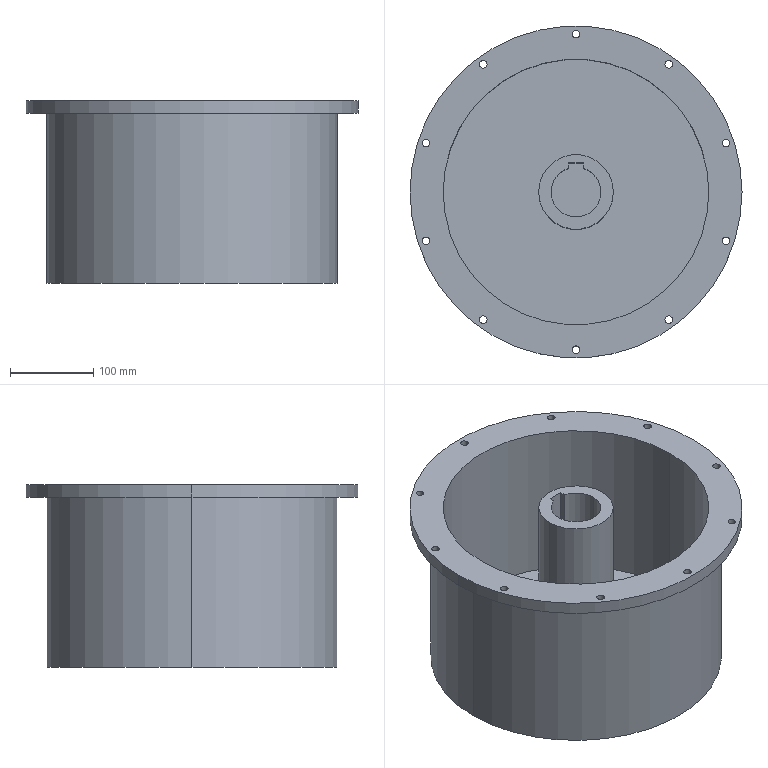Part | SolidWorks | features ICE 4, Extrusion 1 | 1 solid | 40 faces | box 400 x 400 x 220 mm | volume 6200986 mm3 | cylinder 31 | plane 9 | commonest cylinder face diameters 9 x20 60 x3 90 x2 320 x2 350 x2 400 x2
STEP:
#1=CARTESIAN_POINT('',(45.,0.,20.));
#2=VERTEX_POINT('',#1);
#3=CARTESIAN_POINT('',(-45.,0.,20.));
#4=VERTEX_POINT('',#3);
#5=CARTESIAN_POINT('',(0.,0.,20.));
#6=DIRECTION('',(0.,0.,1.));
#7=DIRECTION('',(1.,0.,0.));
#8=AXIS2_PLACEMENT_3D('',#5,#6,#7);
#9=CIRCLE('',#8,45.);
#10=EDGE_CURVE('',#2,#4,#9,.T.);
#11=ORIENTED_EDGE('',*,*,#10,.T.);
#12=CARTESIAN_POINT('',(-45.,0.,220.));
#13=VERTEX_POINT('',#12);
#14=CARTESIAN_POINT('',(-45.,0.,20.));
#15=DIRECTION('',(0.,0.,1.));
#16=VECTOR('',#15,1000.);
#17=LINE('',#14,#16);
#18=EDGE_CURVE('',#4,#13,#17,.T.);
#19=ORIENTED_EDGE('',*,*,#18,.T.);
#20=CARTESIAN_POINT('',(45.,0.,220.));
#21=VERTEX_POINT('',#20);
#22=CARTESIAN_POINT('',(0.,0.,220.));
#23=DIRECTION('',(0.,0.,1.));
#24=DIRECTION('',(1.,0.,0.));
#25=AXIS2_PLACEMENT_3D('',#22,#23,#24);
#26=CIRCLE('',#25,45.);
#27=EDGE_CURVE('',#21,#13,#26,.T.);
#28=ORIENTED_EDGE('',*,*,#27,.F.);
#29=CARTESIAN_POINT('',(45.,0.,20.));
#30=DIRECTION('',(0.,0.,1.));
#31=VECTOR('',#30,1000.);
#32=LINE('',#29,#31);
#33=EDGE_CURVE('',#2,#21,#32,.T.);
#34=ORIENTED_EDGE('',*,*,#33,.F.);
#35=EDGE_LOOP('',(#11,#19,#28,#34));
#36=FACE_OUTER_BOUND('',#35,.T.);
#37=CARTESIAN_POINT('',(0.,0.,20.));
#38=DIRECTION('',(0.,0.,1.));
#39=DIRECTION('',(1.,0.,0.));
#40=AXIS2_PLACEMENT_3D('',#37,#38,#39);
#41=CYLINDRICAL_SURFACE('',#40,45.);
#42=ADVANCED_FACE('',(#36),#41,.T.);
#43=CARTESIAN_POINT('',(-160.,0.,20.));
#44=VERTEX_POINT('',#43);
#45=CARTESIAN_POINT('',(160.,0.,20.));
#46=VERTEX_POINT('',#45);
#47=CARTESIAN_POINT('',(0.,0.,20.));
#48=DIRECTION('',(0.,0.,1.));
#49=DIRECTION('',(1.,0.,0.));
#50=AXIS2_PLACEMENT_3D('',#47,#48,#49);
#51=CIRCLE('',#50,160.);
#52=EDGE_CURVE('',#44,#46,#51,.T.);
#53=ORIENTED_EDGE('',*,*,#52,.F.);
#54=CARTESIAN_POINT('',(-160.,0.,220.));
#55=VERTEX_POINT('',#54);
#56=CARTESIAN_POINT('',(-160.,0.,20.));
#57=DIRECTION('',(0.,0.,1.));
#58=VECTOR('',#57,1000.);
#59=LINE('',#56,#58);
#60=EDGE_CURVE('',#44,#55,#59,.T.);
#61=ORIENTED_EDGE('',*,*,#60,.T.);
#62=CARTESIAN_POINT('',(160.,0.,220.));
#63=VERTEX_POINT('',#62);
#64=CARTESIAN_POINT('',(0.,0.,220.));
#65=DIRECTION('',(0.,0.,1.));
#66=DIRECTION('',(1.,0.,0.));
#67=AXIS2_PLACEMENT_3D('',#64,#65,#66);
#68=CIRCLE('',#67,160.);
#69=EDGE_CURVE('',#55,#63,#68,.T.);
#70=ORIENTED_EDGE('',*,*,#69,.T.);
#71=CARTESIAN_POINT('',(160.,0.,20.));
#72=DIRECTION('',(0.,0.,1.));
#73=VECTOR('',#72,1000.);
#74=LINE('',#71,#73);
#75=EDGE_CURVE('',#46,#63,#74,.T.);
#76=ORIENTED_EDGE('',*,*,#75,.F.);
#77=EDGE_LOOP('',(#53,#61,#70,#76));
#78=FACE_OUTER_BOUND('',#77,.T.);
#79=CARTESIAN_POINT('',(0.,0.,20.));
#80=DIRECTION('',(0.,0.,1.));
#81=DIRECTION('',(1.,0.,0.));
#82=AXIS2_PLACEMENT_3D('',#79,#80,#81);
#83=CYLINDRICAL_SURFACE('',#82,160.);
#84=ADVANCED_FACE('',(#78),#83,.F.);
#85=CARTESIAN_POINT('',(-116.179,153.713,205.));
#86=VERTEX_POINT('',#85);
#87=CARTESIAN_POINT('',(-107.179,153.713,205.));
#88=VERTEX_POINT('',#87);
#89=CARTESIAN_POINT('',(-111.679,153.713,205.));
#90=DIRECTION('',(0.,0.,1.));
#91=DIRECTION('',(1.,0.,0.));
#92=AXIS2_PLACEMENT_3D('',#89,#90,#91);
#93=CIRCLE('',#92,4.5);
#94=EDGE_CURVE('',#86,#88,#93,.T.);
#95=ORIENTED_EDGE('',*,*,#94,.F.);
#96=CARTESIAN_POINT('',(-116.179,153.713,220.));
#97=VERTEX_POINT('',#96);
#98=CARTESIAN_POINT('',(-116.179,153.713,205.));
#99=DIRECTION('',(0.,0.,1.));
#100=VECTOR('',#99,1000.);
#101=LINE('',#98,#100);
#102=EDGE_CURVE('',#86,#97,#101,.T.);
#103=ORIENTED_EDGE('',*,*,#102,.T.);
#104=CARTESIAN_POINT('',(-107.179,153.713,220.));
#105=VERTEX_POINT('',#104);
#106=CARTESIAN_POINT('',(-111.679,153.713,220.));
#107=DIRECTION('',(0.,0.,1.));
#108=DIRECTION('',(1.,0.,0.));
#109=AXIS2_PLACEMENT_3D('',#106,#107,#108);
#110=CIRCLE('',#109,4.5);
#111=EDGE_CURVE('',#97,#105,#110,.T.);
#112=ORIENTED_EDGE('',*,*,#111,.T.);
#113=CARTESIAN_POINT('',(-107.179,153.713,205.));
#114=DIRECTION('',(0.,0.,1.));
#115=VECTOR('',#114,1000.);
#116=LINE('',#113,#115);
#117=EDGE_CURVE('',#88,#105,#116,.T.);
#118=ORIENTED_EDGE('',*,*,#117,.F.);
#119=EDGE_LOOP('',(#95,#103,#112,#118));
#120=FACE_OUTER_BOUND('',#119,.T.);
#121=CARTESIAN_POINT('',(-111.679,153.713,205.));
#122=DIRECTION('',(0.,0.,1.));
#123=DIRECTION('',(1.,0.,0.));
#124=AXIS2_PLACEMENT_3D('',#121,#122,#123);
#125=CYLINDRICAL_SURFACE('',#124,4.5);
#126=ADVANCED_FACE('',(#120),#125,.F.);
#127=CARTESIAN_POINT('',(-185.201,58.713,205.));
#128=VERTEX_POINT('',#127);
#129=CARTESIAN_POINT('',(-176.201,58.713,205.));
#130=VERTEX_POINT('',#129);
#131=CARTESIAN_POINT('',(-180.701,58.713,205.));
#132=DIRECTION('',(0.,0.,1.));
#133=DIRECTION('',(1.,0.,0.));
#134=AXIS2_PLACEMENT_3D('',#131,#132,#133);
#135=CIRCLE('',#134,4.5);
#136=EDGE_CURVE('',#128,#130,#135,.T.);
#137=ORIENTED_EDGE('',*,*,#136,.F.);
#138=CARTESIAN_POINT('',(-185.201,58.713,220.));
#139=VERTEX_POINT('',#138);
#140=CARTESIAN_POINT('',(-185.201,58.713,205.));
#141=DIRECTION('',(0.,0.,1.));
#142=VECTOR('',#141,1000.);
#143=LINE('',#140,#142);
#144=EDGE_CURVE('',#128,#139,#143,.T.);
#145=ORIENTED_EDGE('',*,*,#144,.T.);
#146=CARTESIAN_POINT('',(-176.201,58.713,220.));
#147=VERTEX_POINT('',#146);
#148=CARTESIAN_POINT('',(-180.701,58.713,220.));
#149=DIRECTION('',(0.,0.,1.));
#150=DIRECTION('',(1.,0.,0.));
#151=AXIS2_PLACEMENT_3D('',#148,#149,#150);
#152=CIRCLE('',#151,4.5);
#153=EDGE_CURVE('',#139,#147,#152,.T.);
#154=ORIENTED_EDGE('',*,*,#153,.T.);
#155=CARTESIAN_POINT('',(-176.201,58.713,205.));
#156=DIRECTION('',(0.,0.,1.));
#157=VECTOR('',#156,1000.);
#158=LINE('',#155,#157);
#159=EDGE_CURVE('',#130,#147,#158,.T.);
#160=ORIENTED_EDGE('',*,*,#159,.F.);
#161=EDGE_LOOP('',(#137,#145,#154,#160));
#162=FACE_OUTER_BOUND('',#161,.T.);
#163=CARTESIAN_POINT('',(-180.701,58.713,205.));
#164=DIRECTION('',(0.,0.,1.));
#165=DIRECTION('',(1.,0.,0.));
#166=AXIS2_PLACEMENT_3D('',#163,#164,#165);
#167=CYLINDRICAL_SURFACE('',#166,4.5);
#168=ADVANCED_FACE('',(#162),#167,.F.);
#169=CARTESIAN_POINT('',(-185.201,-58.713,205.));
#170=VERTEX_POINT('',#169);
#171=CARTESIAN_POINT('',(-176.201,-58.713,205.));
#172=VERTEX_POINT('',#171);
#173=CARTESIAN_POINT('',(-180.701,-58.713,205.));
#174=DIRECTION('',(0.,0.,1.));
#175=DIRECTION('',(1.,0.,0.));
#176=AXIS2_PLACEMENT_3D('',#173,#174,#175);
#177=CIRCLE('',#176,4.5);
#178=EDGE_CURVE('',#170,#172,#177,.T.);
#179=ORIENTED_EDGE('',*,*,#178,.F.);
#180=CARTESIAN_POINT('',(-185.201,-58.713,220.));
#181=VERTEX_POINT('',#180);
#182=CARTESIAN_POINT('',(-185.201,-58.713,205.));
#183=DIRECTION('',(0.,0.,1.));
#184=VECTOR('',#183,1000.);
#185=LINE('',#182,#184);
#186=EDGE_CURVE('',#170,#181,#185,.T.);
#187=ORIENTED_EDGE('',*,*,#186,.T.);
#188=CARTESIAN_POINT('',(-176.201,-58.713,220.));
#189=VERTEX_POINT('',#188);
#190=CARTESIAN_POINT('',(-180.701,-58.713,220.));
#191=DIRECTION('',(0.,0.,1.));
#192=DIRECTION('',(1.,0.,0.));
#193=AXIS2_PLACEMENT_3D('',#190,#191,#192);
#194=CIRCLE('',#193,4.5);
#195=EDGE_CURVE('',#181,#189,#194,.T.);
#196=ORIENTED_EDGE('',*,*,#195,.T.);
#197=CARTESIAN_POINT('',(-176.201,-58.713,205.));
#198=DIRECTION('',(0.,0.,1.));
#199=VECTOR('',#198,1000.);
#200=LINE('',#197,#199);
#201=EDGE_CURVE('',#172,#189,#200,.T.);
#202=ORIENTED_EDGE('',*,*,#201,.F.);
#203=EDGE_LOOP('',(#179,#187,#196,#202));
#204=FACE_OUTER_BOUND('',#203,.T.);
#205=CARTESIAN_POINT('',(-180.701,-58.713,205.));
#206=DIRECTION('',(0.,0.,1.));
#207=DIRECTION('',(1.,0.,0.));
#208=AXIS2_PLACEMENT_3D('',#205,#206,#207);
#209=CYLINDRICAL_SURFACE('',#208,4.5);
#210=ADVANCED_FACE('',(#204),#209,.F.);
#211=CARTESIAN_POINT('',(-116.179,-153.713,205.));
#212=VERTEX_POINT('',#211);
#213=CARTESIAN_POINT('',(-107.179,-153.713,205.));
#214=VERTEX_POINT('',#213);
#215=CARTESIAN_POINT('',(-111.679,-153.713,205.));
#216=DIRECTION('',(0.,0.,1.));
#217=DIRECTION('',(1.,0.,0.));
#218=AXIS2_PLACEMENT_3D('',#215,#216,#217);
#219=CIRCLE('',#218,4.5);
#220=EDGE_CURVE('',#212,#214,#219,.T.);
#221=ORIENTED_EDGE('',*,*,#220,.F.);
#222=CARTESIAN_POINT('',(-116.179,-153.713,220.));
#223=VERTEX_POINT('',#222);
#224=CARTESIAN_POINT('',(-116.179,-153.713,205.));
#225=DIRECTION('',(0.,0.,1.));
#226=VECTOR('',#225,1000.);
#227=LINE('',#224,#226);
#228=EDGE_CURVE('',#212,#223,#227,.T.);
#229=ORIENTED_EDGE('',*,*,#228,.T.);
#230=CARTESIAN_POINT('',(-107.179,-153.713,220.));
#231=VERTEX_POINT('',#230);
#232=CARTESIAN_POINT('',(-111.679,-153.713,220.));
#233=DIRECTION('',(0.,0.,1.));
#234=DIRECTION('',(1.,0.,0.));
#235=AXIS2_PLACEMENT_3D('',#232,#233,#234);
#236=CIRCLE('',#235,4.5);
#237=EDGE_CURVE('',#223,#231,#236,.T.);
#238=ORIENTED_EDGE('',*,*,#237,.T.);
#239=CARTESIAN_POINT('',(-107.179,-153.713,205.));
#240=DIRECTION('',(0.,0.,1.));
#241=VECTOR('',#240,1000.);
#242=LINE('',#239,#241);
#243=EDGE_CURVE('',#214,#231,#242,.T.);
#244=ORIENTED_EDGE('',*,*,#243,.F.);
#245=EDGE_LOOP('',(#221,#229,#238,#244));
#246=FACE_OUTER_BOUND('',#245,.T.);
#247=CARTESIAN_POINT('',(-111.679,-153.713,205.));
#248=DIRECTION('',(0.,0.,1.));
#249=DIRECTION('',(1.,0.,0.));
#250=AXIS2_PLACEMENT_3D('',#247,#248,#249);
#251=CYLINDRICAL_SURFACE('',#250,4.5);
#252=ADVANCED_FACE('',(#246),#251,.F.);
#253=CARTESIAN_POINT('',(-4.5,-190.,205.));
#254=VERTEX_POINT('',#253);
#255=CARTESIAN_POINT('',(4.5,-190.,205.));
#256=VERTEX_POINT('',#255);
#257=CARTESIAN_POINT('',(0.,-190.,205.));
#258=DIRECTION('',(0.,0.,1.));
#259=DIRECTION('',(1.,0.,0.));
#260=AXIS2_PLACEMENT_3D('',#257,#258,#259);
#261=CIRCLE('',#260,4.5);
#262=EDGE_CURVE('',#254,#256,#261,.T.);
#263=ORIENTED_EDGE('',*,*,#262,.F.);
#264=CARTESIAN_POINT('',(-4.5,-190.,220.));
#265=VERTEX_POINT('',#264);
#266=CARTESIAN_POINT('',(-4.5,-190.,205.));
#267=DIRECTION('',(0.,0.,1.));
#268=VECTOR('',#267,1000.);
#269=LINE('',#266,#268);
#270=EDGE_CURVE('',#254,#265,#269,.T.);
#271=ORIENTED_EDGE('',*,*,#270,.T.);
#272=CARTESIAN_POINT('',(4.5,-190.,220.));
#273=VERTEX_POINT('',#272);
#274=CARTESIAN_POINT('',(0.,-190.,220.));
#275=DIRECTION('',(0.,0.,1.));
#276=DIRECTION('',(1.,0.,0.));
#277=AXIS2_PLACEMENT_3D('',#274,#275,#276);
#278=CIRCLE('',#277,4.5);
#279=EDGE_CURVE('',#265,#273,#278,.T.);
#280=ORIENTED_EDGE('',*,*,#279,.T.);
#281=CARTESIAN_POINT('',(4.5,-190.,205.));
#282=DIRECTION('',(0.,0.,1.));
#283=VECTOR('',#282,1000.);
#284=LINE('',#281,#283);
#285=EDGE_CURVE('',#256,#273,#284,.T.);
#286=ORIENTED_EDGE('',*,*,#285,.F.);
#287=EDGE_LOOP('',(#263,#271,#280,#286));
#288=FACE_OUTER_BOUND('',#287,.T.);
#289=CARTESIAN_POINT('',(0.,-190.,205.));
#290=DIRECTION('',(0.,0.,1.));
#291=DIRECTION('',(1.,0.,0.));
#292=AXIS2_PLACEMENT_3D('',#289,#290,#291);
#293=CYLINDRICAL_SURFACE('',#292,4.5);
#294=ADVANCED_FACE('',(#288),#293,.F.);
#295=CARTESIAN_POINT('',(107.179,-153.713,205.));
#296=VERTEX_POINT('',#295);
#297=CARTESIAN_POINT('',(116.179,-153.713,205.));
#298=VERTEX_POINT('',#297);
#299=CARTESIAN_POINT('',(111.679,-153.713,205.));
#300=DIRECTION('',(0.,0.,1.));
#301=DIRECTION('',(1.,0.,0.));
#302=AXIS2_PLACEMENT_3D('',#299,#300,#301);
#303=CIRCLE('',#302,4.5);
#304=EDGE_CURVE('',#296,#298,#303,.T.);
#305=ORIENTED_EDGE('',*,*,#304,.F.);
#306=CARTESIAN_POINT('',(107.179,-153.713,220.));
#307=VERTEX_POINT('',#306);
#308=CARTESIAN_POINT('',(107.179,-153.713,205.));
#309=DIRECTION('',(0.,0.,1.));
#310=VECTOR('',#309,1000.);
#311=LINE('',#308,#310);
#312=EDGE_CURVE('',#296,#307,#311,.T.);
#313=ORIENTED_EDGE('',*,*,#312,.T.);
#314=CARTESIAN_POINT('',(116.179,-153.713,220.));
#315=VERTEX_POINT('',#314);
#316=CARTESIAN_POINT('',(111.679,-153.713,220.));
#317=DIRECTION('',(0.,0.,1.));
#318=DIRECTION('',(1.,0.,0.));
#319=AXIS2_PLACEMENT_3D('',#316,#317,#318);
#320=CIRCLE('',#319,4.5);
#321=EDGE_CURVE('',#307,#315,#320,.T.);
#322=ORIENTED_EDGE('',*,*,#321,.T.);
#323=CARTESIAN_POINT('',(116.179,-153.713,205.));
#324=DIRECTION('',(0.,0.,1.));
#325=VECTOR('',#324,1000.);
#326=LINE('',#323,#325);
#327=EDGE_CURVE('',#298,#315,#326,.T.);
#328=ORIENTED_EDGE('',*,*,#327,.F.);
#329=EDGE_LOOP('',(#305,#313,#322,#328));
#330=FACE_OUTER_BOUND('',#329,.T.);
#331=CARTESIAN_POINT('',(111.679,-153.713,205.));
#332=DIRECTION('',(0.,0.,1.));
#333=DIRECTION('',(1.,0.,0.));
#334=AXIS2_PLACEMENT_3D('',#331,#332,#333);
#335=CYLINDRICAL_SURFACE('',#334,4.5);
#336=ADVANCED_FACE('',(#330),#335,.F.);
#337=CARTESIAN_POINT('',(176.201,-58.713,205.));
#338=VERTEX_POINT('',#337);
#339=CARTESIAN_POINT('',(185.201,-58.713,205.));
#340=VERTEX_POINT('',#339);
#341=CARTESIAN_POINT('',(180.701,-58.713,205.));
#342=DIRECTION('',(0.,0.,1.));
#343=DIRECTION('',(1.,0.,0.));
#344=AXIS2_PLACEMENT_3D('',#341,#342,#343);
#345=CIRCLE('',#344,4.5);
#346=EDGE_CURVE('',#338,#340,#345,.T.);
#347=ORIENTED_EDGE('',*,*,#346,.F.);
#348=CARTESIAN_POINT('',(176.201,-58.713,220.));
#349=VERTEX_POINT('',#348);
#350=CARTESIAN_POINT('',(176.201,-58.713,205.));
#351=DIRECTION('',(0.,0.,1.));
#352=VECTOR('',#351,1000.);
#353=LINE('',#350,#352);
#354=EDGE_CURVE('',#338,#349,#353,.T.);
#355=ORIENTED_EDGE('',*,*,#354,.T.);
#356=CARTESIAN_POINT('',(185.201,-58.713,220.));
#357=VERTEX_POINT('',#356);
#358=CARTESIAN_POINT('',(180.701,-58.713,220.));
#359=DIRECTION('',(0.,0.,1.));
#360=DIRECTION('',(1.,0.,0.));
#361=AXIS2_PLACEMENT_3D('',#358,#359,#360);
#362=CIRCLE('',#361,4.5);
#363=EDGE_CURVE('',#349,#357,#362,.T.);
#364=ORIENTED_EDGE('',*,*,#363,.T.);
#365=CARTESIAN_POINT('',(185.201,-58.713,205.));
#366=DIRECTION('',(0.,0.,1.));
#367=VECTOR('',#366,1000.);
#368=LINE('',#365,#367);
#369=EDGE_CURVE('',#340,#357,#368,.T.);
#370=ORIENTED_EDGE('',*,*,#369,.F.);
#371=EDGE_LOOP('',(#347,#355,#364,#370));
#372=FACE_OUTER_BOUND('',#371,.T.);
#373=CARTESIAN_POINT('',(180.701,-58.713,205.));
#374=DIRECTION('',(0.,0.,1.));
#375=DIRECTION('',(1.,0.,0.));
#376=AXIS2_PLACEMENT_3D('',#373,#374,#375);
#377=CYLINDRICAL_SURFACE('',#376,4.5);
#378=ADVANCED_FACE('',(#372),#377,.F.);
#379=CARTESIAN_POINT('',(176.201,58.713,205.));
#380=VERTEX_POINT('',#379);
#381=CARTESIAN_POINT('',(185.201,58.713,205.));
#382=VERTEX_POINT('',#381);
#383=CARTESIAN_POINT('',(180.701,58.713,205.));
#384=DIRECTION('',(0.,0.,1.));
#385=DIRECTION('',(1.,0.,0.));
#386=AXIS2_PLACEMENT_3D('',#383,#384,#385);
#387=CIRCLE('',#386,4.5);
#388=EDGE_CURVE('',#380,#382,#387,.T.);
#389=ORIENTED_EDGE('',*,*,#388,.F.);
#390=CARTESIAN_POINT('',(176.201,58.713,220.));
#391=VERTEX_POINT('',#390);
#392=CARTESIAN_POINT('',(176.201,58.713,205.));
#393=DIRECTION('',(0.,0.,1.));
#394=VECTOR('',#393,1000.);
#395=LINE('',#392,#394);
#396=EDGE_CURVE('',#380,#391,#395,.T.);
#397=ORIENTED_EDGE('',*,*,#396,.T.);
#398=CARTESIAN_POINT('',(185.201,58.713,220.));
#399=VERTEX_POINT('',#398);
#400=CARTESIAN_POINT('',(180.701,58.713,220.));
#401=DIRECTION('',(0.,0.,1.));
#402=DIRECTION('',(1.,0.,0.));
#403=AXIS2_PLACEMENT_3D('',#400,#401,#402);
#404=CIRCLE('',#403,4.5);
#405=EDGE_CURVE('',#391,#399,#404,.T.);
#406=ORIENTED_EDGE('',*,*,#405,.T.);
#407=CARTESIAN_POINT('',(185.201,58.713,205.));
#408=DIRECTION('',(0.,0.,1.));
#409=VECTOR('',#408,1000.);
#410=LINE('',#407,#409);
#411=EDGE_CURVE('',#382,#399,#410,.T.);
#412=ORIENTED_EDGE('',*,*,#411,.F.);
#413=EDGE_LOOP('',(#389,#397,#406,#412));
#414=FACE_OUTER_BOUND('',#413,.T.);
#415=CARTESIAN_POINT('',(180.701,58.713,205.));
#416=DIRECTION('',(0.,0.,1.));
#417=DIRECTION('',(1.,0.,0.));
#418=AXIS2_PLACEMENT_3D('',#415,#416,#417);
#419=CYLINDRICAL_SURFACE('',#418,4.5);
#420=ADVANCED_FACE('',(#414),#419,.F.);
#421=CARTESIAN_POINT('',(107.179,153.713,205.));
#422=VERTEX_POINT('',#421);
#423=CARTESIAN_POINT('',(116.179,153.713,205.));
#424=VERTEX_POINT('',#423);
#425=CARTESIAN_POINT('',(111.679,153.713,205.));
#426=DIRECTION('',(0.,0.,1.));
#427=DIRECTION('',(1.,0.,0.));
#428=AXIS2_PLACEMENT_3D('',#425,#426,#427);
#429=CIRCLE('',#428,4.5);
#430=EDGE_CURVE('',#422,#424,#429,.T.);
#431=ORIENTED_EDGE('',*,*,#430,.F.);
#432=CARTESIAN_POINT('',(107.179,153.713,220.));
#433=VERTEX_POINT('',#432);
#434=CARTESIAN_POINT('',(107.179,153.713,205.));
#435=DIRECTION('',(0.,0.,1.));
#436=VECTOR('',#435,1000.);
#437=LINE('',#434,#436);
#438=EDGE_CURVE('',#422,#433,#437,.T.);
#439=ORIENTED_EDGE('',*,*,#438,.T.);
#440=CARTESIAN_POINT('',(116.179,153.713,220.));
#441=VERTEX_POINT('',#440);
#442=CARTESIAN_POINT('',(111.679,153.713,220.));
#443=DIRECTION('',(0.,0.,1.));
#444=DIRECTION('',(1.,0.,0.));
#445=AXIS2_PLACEMENT_3D('',#442,#443,#444);
#446=CIRCLE('',#445,4.5);
#447=EDGE_CURVE('',#433,#441,#446,.T.);
#448=ORIENTED_EDGE('',*,*,#447,.T.);
#449=CARTESIAN_POINT('',(116.179,153.713,205.));
#450=DIRECTION('',(0.,0.,1.));
#451=VECTOR('',#450,1000.);
#452=LINE('',#449,#451);
#453=EDGE_CURVE('',#424,#441,#452,.T.);
#454=ORIENTED_EDGE('',*,*,#453,.F.);
#455=EDGE_LOOP('',(#431,#439,#448,#454));
#456=FACE_OUTER_BOUND('',#455,.T.);
#457=CARTESIAN_POINT('',(111.679,153.713,205.));
#458=DIRECTION('',(0.,0.,1.));
#459=DIRECTION('',(1.,0.,0.));
#460=AXIS2_PLACEMENT_3D('',#457,#458,#459);
#461=CYLINDRICAL_SURFACE('',#460,4.5);
#462=ADVANCED_FACE('',(#456),#461,.F.);
#463=CARTESIAN_POINT('',(-4.5,190.,205.));
#464=VERTEX_POINT('',#463);
#465=CARTESIAN_POINT('',(4.5,190.,205.));
#466=VERTEX_POINT('',#465);
#467=CARTESIAN_POINT('',(0.,190.,205.));
#468=DIRECTION('',(0.,0.,1.));
#469=DIRECTION('',(1.,0.,0.));
#470=AXIS2_PLACEMENT_3D('',#467,#468,#469);
#471=CIRCLE('',#470,4.5);
#472=EDGE_CURVE('',#464,#466,#471,.T.);
#473=ORIENTED_EDGE('',*,*,#472,.F.);
#474=CARTESIAN_POINT('',(-4.5,190.,220.));
#475=VERTEX_POINT('',#474);
#476=CARTESIAN_POINT('',(-4.5,190.,205.));
#477=DIRECTION('',(0.,0.,1.));
#478=VECTOR('',#477,1000.);
#479=LINE('',#476,#478);
#480=EDGE_CURVE('',#464,#475,#479,.T.);
#481=ORIENTED_EDGE('',*,*,#480,.T.);
#482=CARTESIAN_POINT('',(4.5,190.,220.));
#483=VERTEX_POINT('',#482);
#484=CARTESIAN_POINT('',(0.,190.,220.));
#485=DIRECTION('',(0.,0.,1.));
#486=DIRECTION('',(1.,0.,0.));
#487=AXIS2_PLACEMENT_3D('',#484,#485,#486);
#488=CIRCLE('',#487,4.5);
#489=EDGE_CURVE('',#475,#483,#488,.T.);
#490=ORIENTED_EDGE('',*,*,#489,.T.);
#491=CARTESIAN_POINT('',(4.5,190.,205.));
#492=DIRECTION('',(0.,0.,1.));
#493=VECTOR('',#492,1000.);
#494=LINE('',#491,#493);
#495=EDGE_CURVE('',#466,#483,#494,.T.);
#496=ORIENTED_EDGE('',*,*,#495,.F.);
#497=EDGE_LOOP('',(#473,#481,#490,#496));
#498=FACE_OUTER_BOUND('',#497,.T.);
#499=CARTESIAN_POINT('',(0.,190.,205.));
#500=DIRECTION('',(0.,0.,1.));
#501=DIRECTION('',(1.,0.,0.));
#502=AXIS2_PLACEMENT_3D('',#499,#500,#501);
#503=CYLINDRICAL_SURFACE('',#502,4.5);
#504=ADVANCED_FACE('',(#498),#503,.F.);
#505=CARTESIAN_POINT('',(200.,0.,205.));
#506=VERTEX_POINT('',#505);
#507=CARTESIAN_POINT('',(-200.,0.,205.));
#508=VERTEX_POINT('',#507);
#509=CARTESIAN_POINT('',(0.,0.,205.));
#510=DIRECTION('',(0.,0.,1.));
#511=DIRECTION('',(1.,0.,0.));
#512=AXIS2_PLACEMENT_3D('',#509,#510,#511);
#513=CIRCLE('',#512,200.);
#514=EDGE_CURVE('',#506,#508,#513,.T.);
#515=ORIENTED_EDGE('',*,*,#514,.T.);
#516=CARTESIAN_POINT('',(-200.,0.,220.));
#517=VERTEX_POINT('',#516);
#518=CARTESIAN_POINT('',(-200.,0.,205.));
#519=DIRECTION('',(0.,0.,1.));
#520=VECTOR('',#519,1000.);
#521=LINE('',#518,#520);
#522=EDGE_CURVE('',#508,#517,#521,.T.);
#523=ORIENTED_EDGE('',*,*,#522,.T.);
#524=CARTESIAN_POINT('',(200.,0.,220.));
#525=VERTEX_POINT('',#524);
#526=CARTESIAN_POINT('',(0.,0.,220.));
#527=DIRECTION('',(0.,0.,1.));
#528=DIRECTION('',(1.,0.,0.));
#529=AXIS2_PLACEMENT_3D('',#526,#527,#528);
#530=CIRCLE('',#529,200.);
#531=EDGE_CURVE('',#525,#517,#530,.T.);
#532=ORIENTED_EDGE('',*,*,#531,.F.);
#533=CARTESIAN_POINT('',(200.,0.,205.));
#534=DIRECTION('',(0.,0.,1.));
#535=VECTOR('',#534,1000.);
#536=LINE('',#533,#535);
#537=EDGE_CURVE('',#506,#525,#536,.T.);
#538=ORIENTED_EDGE('',*,*,#537,.F.);
#539=EDGE_LOOP('',(#515,#523,#532,#538));
#540=FACE_OUTER_BOUND('',#539,.T.);
#541=CARTESIAN_POINT('',(0.,0.,205.));
#542=DIRECTION('',(0.,0.,1.));
#543=DIRECTION('',(1.,0.,0.));
#544=AXIS2_PLACEMENT_3D('',#541,#542,#543);
#545=CYLINDRICAL_SURFACE('',#544,200.);
#546=ADVANCED_FACE('',(#540),#545,.T.);
#547=CARTESIAN_POINT('',(175.,0.,205.));
#548=VERTEX_POINT('',#547);
#549=CARTESIAN_POINT('',(-175.,0.,205.));
#550=VERTEX_POINT('',#549);
#551=CARTESIAN_POINT('',(0.,0.,205.));
#552=DIRECTION('',(0.,0.,1.));
#553=DIRECTION('',(1.,0.,0.));
#554=AXIS2_PLACEMENT_3D('',#551,#552,#553);
#555=CIRCLE('',#554,175.);
#556=EDGE_CURVE('',#548,#550,#555,.T.);
#557=ORIENTED_EDGE('',*,*,#556,.F.);
#558=CARTESIAN_POINT('',(175.,0.,0.));
#559=VERTEX_POINT('',#558);
#560=CARTESIAN_POINT('',(175.,0.,220.));
#561=DIRECTION('',(0.,0.,-1.));
#562=VECTOR('',#561,1000.);
#563=LINE('',#560,#562);
#564=EDGE_CURVE('',#548,#559,#563,.T.);
#565=ORIENTED_EDGE('',*,*,#564,.T.);
#566=CARTESIAN_POINT('',(-175.,0.,0.));
#567=VERTEX_POINT('',#566);
#568=CARTESIAN_POINT('',(0.,0.,0.));
#569=DIRECTION('',(0.,0.,1.));
#570=DIRECTION('',(1.,0.,0.));
#571=AXIS2_PLACEMENT_3D('',#568,#569,#570);
#572=CIRCLE('',#571,175.);
#573=EDGE_CURVE('',#559,#567,#572,.T.);
#574=ORIENTED_EDGE('',*,*,#573,.T.);
#575=CARTESIAN_POINT('',(-175.,0.,220.));
#576=DIRECTION('',(0.,0.,-1.));
#577=VECTOR('',#576,1000.);
#578=LINE('',#575,#577);
#579=EDGE_CURVE('',#550,#567,#578,.T.);
#580=ORIENTED_EDGE('',*,*,#579,.F.);
#581=EDGE_LOOP('',(#557,#565,#574,#580));
#582=FACE_OUTER_BOUND('',#581,.T.);
#583=CARTESIAN_POINT('',(0.,0.,220.));
#584=DIRECTION('',(0.,0.,-1.));
#585=DIRECTION('',(-1.,0.,0.));
#586=AXIS2_PLACEMENT_3D('',#583,#584,#585);
#587=CYLINDRICAL_SURFACE('',#586,175.);
#588=ADVANCED_FACE('',(#582),#587,.T.);
#589=CARTESIAN_POINT('',(-30.,0.,220.));
#590=VERTEX_POINT('',#589);
#591=CARTESIAN_POINT('',(30.,0.,220.));
#592=VERTEX_POINT('',#591);
#593=CARTESIAN_POINT('',(0.,0.,220.));
#594=DIRECTION('',(0.,0.,1.));
#595=DIRECTION('',(1.,0.,0.));
#596=AXIS2_PLACEMENT_3D('',#593,#594,#595);
#597=CIRCLE('',#596,30.);
#598=EDGE_CURVE('',#590,#592,#597,.T.);
#599=ORIENTED_EDGE('',*,*,#598,.T.);
#600=CARTESIAN_POINT('',(30.,0.,20.));
#601=VERTEX_POINT('',#600);
#602=CARTESIAN_POINT('',(30.,0.,220.));
#603=DIRECTION('',(0.,0.,-1.));
#604=VECTOR('',#603,1000.);
#605=LINE('',#602,#604);
#606=EDGE_CURVE('',#592,#601,#605,.T.);
#607=ORIENTED_EDGE('',*,*,#606,.T.);
#608=CARTESIAN_POINT('',(-30.,0.,20.));
#609=VERTEX_POINT('',#608);
#610=CARTESIAN_POINT('',(0.,0.,20.));
#611=DIRECTION('',(0.,0.,-1.));
#612=DIRECTION('',(-1.,0.,0.));
#613=AXIS2_PLACEMENT_3D('',#610,#611,#612);
#614=CIRCLE('',#613,30.);
#615=EDGE_CURVE('',#601,#609,#614,.T.);
#616=ORIENTED_EDGE('',*,*,#615,.T.);
#617=CARTESIAN_POINT('',(-30.,0.,220.));
#618=DIRECTION('',(0.,0.,-1.));
#619=VECTOR('',#618,1000.);
#620=LINE('',#617,#619);
#621=EDGE_CURVE('',#590,#609,#620,.T.);
#622=ORIENTED_EDGE('',*,*,#621,.F.);
#623=EDGE_LOOP('',(#599,#607,#616,#622));
#624=FACE_OUTER_BOUND('',#623,.T.);
#625=CARTESIAN_POINT('',(0.,0.,220.));
#626=DIRECTION('',(0.,0.,-1.));
#627=DIRECTION('',(-1.,0.,0.));
#628=AXIS2_PLACEMENT_3D('',#625,#626,#627);
#629=CYLINDRICAL_SURFACE('',#628,30.);
#630=ADVANCED_FACE('',(#624),#629,.F.);
#631=CARTESIAN_POINT('',(-9.,28.618,220.));
#632=VERTEX_POINT('',#631);
#633=CARTESIAN_POINT('',(0.,0.,220.));
#634=DIRECTION('',(0.,0.,1.));
#635=DIRECTION('',(1.,0.,0.));
#636=AXIS2_PLACEMENT_3D('',#633,#634,#635);
#637=CIRCLE('',#636,30.);
#638=EDGE_CURVE('',#632,#590,#637,.T.);
#639=ORIENTED_EDGE('',*,*,#638,.T.);
#640=ORIENTED_EDGE('',*,*,#621,.T.);
#641=CARTESIAN_POINT('',(-9.,28.618,20.));
#642=VERTEX_POINT('',#641);
#643=CARTESIAN_POINT('',(0.,0.,20.));
#644=DIRECTION('',(0.,0.,-1.));
#645=DIRECTION('',(-1.,0.,0.));
#646=AXIS2_PLACEMENT_3D('',#643,#644,#645);
#647=CIRCLE('',#646,30.);
#648=EDGE_CURVE('',#609,#642,#647,.T.);
#649=ORIENTED_EDGE('',*,*,#648,.T.);
#650=CARTESIAN_POINT('',(-9.,28.618,220.));
#651=DIRECTION('',(0.,0.,-1.));
#652=VECTOR('',#651,1000.);
#653=LINE('',#650,#652);
#654=EDGE_CURVE('',#632,#642,#653,.T.);
#655=ORIENTED_EDGE('',*,*,#654,.F.);
#656=EDGE_LOOP('',(#639,#640,#649,#655));
#657=FACE_OUTER_BOUND('',#656,.T.);
#658=CARTESIAN_POINT('',(0.,0.,220.));
#659=DIRECTION('',(0.,0.,-1.));
#660=DIRECTION('',(-1.,0.,0.));
#661=AXIS2_PLACEMENT_3D('',#658,#659,#660);
#662=CYLINDRICAL_SURFACE('',#661,30.);
#663=ADVANCED_FACE('',(#657),#662,.F.);
#664=ORIENTED_EDGE('',*,*,#606,.F.);
#665=CARTESIAN_POINT('',(9.,28.618,220.));
#666=VERTEX_POINT('',#665);
#667=CARTESIAN_POINT('',(0.,0.,220.));
#668=DIRECTION('',(0.,0.,1.));
#669=DIRECTION('',(1.,0.,0.));
#670=AXIS2_PLACEMENT_3D('',#667,#668,#669);
#671=CIRCLE('',#670,30.);
#672=EDGE_CURVE('',#592,#666,#671,.T.);
#673=ORIENTED_EDGE('',*,*,#672,.T.);
#674=CARTESIAN_POINT('',(9.,28.618,20.));
#675=VERTEX_POINT('',#674);
#676=CARTESIAN_POINT('',(9.,28.618,220.));
#677=DIRECTION('',(0.,0.,1.));
#678=VECTOR('',#677,1000.);
#679=LINE('',#676,#678);
#680=EDGE_CURVE('',#675,#666,#679,.T.);
#681=ORIENTED_EDGE('',*,*,#680,.F.);
#682=CARTESIAN_POINT('',(0.,0.,20.));
#683=DIRECTION('',(0.,0.,-1.));
#684=DIRECTION('',(-1.,0.,0.));
#685=AXIS2_PLACEMENT_3D('',#682,#683,#684);
#686=CIRCLE('',#685,30.);
#687=EDGE_CURVE('',#675,#601,#686,.T.);
#688=ORIENTED_EDGE('',*,*,#687,.T.);
#689=EDGE_LOOP('',(#664,#673,#681,#688));
#690=FACE_OUTER_BOUND('',#689,.T.);
#691=CARTESIAN_POINT('',(0.,0.,220.));
#692=DIRECTION('',(0.,0.,-1.));
#693=DIRECTION('',(-1.,0.,0.));
#694=AXIS2_PLACEMENT_3D('',#691,#692,#693);
#695=CYLINDRICAL_SURFACE('',#694,30.);
#696=ADVANCED_FACE('',(#690),#695,.F.);
#697=CARTESIAN_POINT('',(-9.,35.,220.));
#698=VERTEX_POINT('',#697);
#699=CARTESIAN_POINT('',(-9.,35.,220.));
#700=DIRECTION('',(0.,-1.,0.));
#701=VECTOR('',#700,1000.);
#702=LINE('',#699,#701);
#703=EDGE_CURVE('',#698,#632,#702,.T.);
#704=ORIENTED_EDGE('',*,*,#703,.F.);
#705=CARTESIAN_POINT('',(9.,35.,220.));
#706=VERTEX_POINT('',#705);
#707=CARTESIAN_POINT('',(-9.,35.,220.));
#708=DIRECTION('',(-1.,0.,0.));
#709=VECTOR('',#708,1000.);
#710=LINE('',#707,#709);
#711=EDGE_CURVE('',#706,#698,#710,.T.);
#712=ORIENTED_EDGE('',*,*,#711,.F.);
#713=CARTESIAN_POINT('',(9.,35.,220.));
#714=DIRECTION('',(0.,1.,0.));
#715=VECTOR('',#714,1000.);
#716=LINE('',#713,#715);
#717=EDGE_CURVE('',#666,#706,#716,.T.);
#718=ORIENTED_EDGE('',*,*,#717,.F.);
#719=ORIENTED_EDGE('',*,*,#672,.F.);
#720=ORIENTED_EDGE('',*,*,#598,.F.);
#721=ORIENTED_EDGE('',*,*,#638,.F.);
#722=EDGE_LOOP('',(#704,#712,#718,#719,#720,#721));
#723=FACE_BOUND('',#722,.T.);
#724=ORIENTED_EDGE('',*,*,#27,.T.);
#725=CARTESIAN_POINT('',(0.,0.,220.));
#726=DIRECTION('',(0.,0.,1.));
#727=DIRECTION('',(1.,0.,0.));
#728=AXIS2_PLACEMENT_3D('',#725,#726,#727);
#729=CIRCLE('',#728,45.);
#730=EDGE_CURVE('',#13,#21,#729,.T.);
#731=ORIENTED_EDGE('',*,*,#730,.T.);
#732=EDGE_LOOP('',(#724,#731));
#733=FACE_OUTER_BOUND('',#732,.T.);
#734=CARTESIAN_POINT('',(0.,0.,220.));
#735=DIRECTION('',(0.,0.,1.));
#736=DIRECTION('',(1.,0.,0.));
#737=AXIS2_PLACEMENT_3D('',#734,#735,#736);
#738=PLANE('',#737);
#739=ADVANCED_FACE('',(#723,#733),#738,.T.);
#740=ORIENTED_EDGE('',*,*,#564,.F.);
#741=CARTESIAN_POINT('',(0.,0.,205.));
#742=DIRECTION('',(0.,0.,1.));
#743=DIRECTION('',(1.,0.,0.));
#744=AXIS2_PLACEMENT_3D('',#741,#742,#743);
#745=CIRCLE('',#744,175.);
#746=EDGE_CURVE('',#550,#548,#745,.T.);
#747=ORIENTED_EDGE('',*,*,#746,.F.);
#748=ORIENTED_EDGE('',*,*,#579,.T.);
#749=CARTESIAN_POINT('',(0.,0.,0.));
#750=DIRECTION('',(0.,0.,1.));
#751=DIRECTION('',(1.,0.,0.));
#752=AXIS2_PLACEMENT_3D('',#749,#750,#751);
#753=CIRCLE('',#752,175.);
#754=EDGE_CURVE('',#567,#559,#753,.T.);
#755=ORIENTED_EDGE('',*,*,#754,.T.);
#756=EDGE_LOOP('',(#740,#747,#748,#755));
#757=FACE_OUTER_BOUND('',#756,.T.);
#758=CARTESIAN_POINT('',(0.,0.,220.));
#759=DIRECTION('',(0.,0.,-1.));
#760=DIRECTION('',(-1.,0.,0.));
#761=AXIS2_PLACEMENT_3D('',#758,#759,#760);
#762=CYLINDRICAL_SURFACE('',#761,175.);
#763=ADVANCED_FACE('',(#757),#762,.T.);
#764=CARTESIAN_POINT('',(0.,0.,220.));
#765=DIRECTION('',(0.,0.,1.));
#766=DIRECTION('',(1.,0.,0.));
#767=AXIS2_PLACEMENT_3D('',#764,#765,#766);
#768=CIRCLE('',#767,160.);
#769=EDGE_CURVE('',#63,#55,#768,.T.);
#770=ORIENTED_EDGE('',*,*,#769,.F.);
#771=ORIENTED_EDGE('',*,*,#69,.F.);
#772=EDGE_LOOP('',(#770,#771));
#773=FACE_BOUND('',#772,.T.);
#774=ORIENTED_EDGE('',*,*,#531,.T.);
#775=CARTESIAN_POINT('',(0.,0.,220.));
#776=DIRECTION('',(0.,0.,1.));
#777=DIRECTION('',(1.,0.,0.));
#778=AXIS2_PLACEMENT_3D('',#775,#776,#777);
#779=CIRCLE('',#778,200.);
#780=EDGE_CURVE('',#517,#525,#779,.T.);
#781=ORIENTED_EDGE('',*,*,#780,.T.);
#782=EDGE_LOOP('',(#774,#781));
#783=FACE_OUTER_BOUND('',#782,.T.);
#784=CARTESIAN_POINT('',(0.,190.,220.));
#785=DIRECTION('',(0.,0.,1.));
#786=DIRECTION('',(1.,0.,0.));
#787=AXIS2_PLACEMENT_3D('',#784,#785,#786);
#788=CIRCLE('',#787,4.5);
#789=EDGE_CURVE('',#483,#475,#788,.T.);
#790=ORIENTED_EDGE('',*,*,#789,.F.);
#791=ORIENTED_EDGE('',*,*,#489,.F.);
#792=EDGE_LOOP('',(#790,#791));
#793=FACE_BOUND('',#792,.T.);
#794=CARTESIAN_POINT('',(111.679,153.713,220.));
#795=DIRECTION('',(0.,0.,1.));
#796=DIRECTION('',(1.,0.,0.));
#797=AXIS2_PLACEMENT_3D('',#794,#795,#796);
#798=CIRCLE('',#797,4.5);
#799=EDGE_CURVE('',#441,#433,#798,.T.);
#800=ORIENTED_EDGE('',*,*,#799,.F.);
#801=ORIENTED_EDGE('',*,*,#447,.F.);
#802=EDGE_LOOP('',(#800,#801));
#803=FACE_BOUND('',#802,.T.);
#804=CARTESIAN_POINT('',(180.701,58.713,220.));
#805=DIRECTION('',(0.,0.,1.));
#806=DIRECTION('',(1.,0.,0.));
#807=AXIS2_PLACEMENT_3D('',#804,#805,#806);
#808=CIRCLE('',#807,4.5);
#809=EDGE_CURVE('',#399,#391,#808,.T.);
#810=ORIENTED_EDGE('',*,*,#809,.F.);
#811=ORIENTED_EDGE('',*,*,#405,.F.);
#812=EDGE_LOOP('',(#810,#811));
#813=FACE_BOUND('',#812,.T.);
#814=CARTESIAN_POINT('',(180.701,-58.713,220.));
#815=DIRECTION('',(0.,0.,1.));
#816=DIRECTION('',(1.,0.,0.));
#817=AXIS2_PLACEMENT_3D('',#814,#815,#816);
#818=CIRCLE('',#817,4.5);
#819=EDGE_CURVE('',#357,#349,#818,.T.);
#820=ORIENTED_EDGE('',*,*,#819,.F.);
#821=ORIENTED_EDGE('',*,*,#363,.F.);
#822=EDGE_LOOP('',(#820,#821));
#823=FACE_BOUND('',#822,.T.);
#824=CARTESIAN_POINT('',(111.679,-153.713,220.));
#825=DIRECTION('',(0.,0.,1.));
#826=DIRECTION('',(1.,0.,0.));
#827=AXIS2_PLACEMENT_3D('',#824,#825,#826);
#828=CIRCLE('',#827,4.5);
#829=EDGE_CURVE('',#315,#307,#828,.T.);
#830=ORIENTED_EDGE('',*,*,#829,.F.);
#831=ORIENTED_EDGE('',*,*,#321,.F.);
#832=EDGE_LOOP('',(#830,#831));
#833=FACE_BOUND('',#832,.T.);
#834=CARTESIAN_POINT('',(0.,-190.,220.));
#835=DIRECTION('',(0.,0.,1.));
#836=DIRECTION('',(1.,0.,0.));
#837=AXIS2_PLACEMENT_3D('',#834,#835,#836);
#838=CIRCLE('',#837,4.5);
#839=EDGE_CURVE('',#273,#265,#838,.T.);
#840=ORIENTED_EDGE('',*,*,#839,.F.);
#841=ORIENTED_EDGE('',*,*,#279,.F.);
#842=EDGE_LOOP('',(#840,#841));
#843=FACE_BOUND('',#842,.T.);
#844=CARTESIAN_POINT('',(-111.679,-153.713,220.));
#845=DIRECTION('',(0.,0.,1.));
#846=DIRECTION('',(1.,0.,0.));
#847=AXIS2_PLACEMENT_3D('',#844,#845,#846);
#848=CIRCLE('',#847,4.5);
#849=EDGE_CURVE('',#231,#223,#848,.T.);
#850=ORIENTED_EDGE('',*,*,#849,.F.);
#851=ORIENTED_EDGE('',*,*,#237,.F.);
#852=EDGE_LOOP('',(#850,#851));
#853=FACE_BOUND('',#852,.T.);
#854=CARTESIAN_POINT('',(-180.701,-58.713,220.));
#855=DIRECTION('',(0.,0.,1.));
#856=DIRECTION('',(1.,0.,0.));
#857=AXIS2_PLACEMENT_3D('',#854,#855,#856);
#858=CIRCLE('',#857,4.5);
#859=EDGE_CURVE('',#189,#181,#858,.T.);
#860=ORIENTED_EDGE('',*,*,#859,.F.);
#861=ORIENTED_EDGE('',*,*,#195,.F.);
#862=EDGE_LOOP('',(#860,#861));
#863=FACE_BOUND('',#862,.T.);
#864=CARTESIAN_POINT('',(-180.701,58.713,220.));
#865=DIRECTION('',(0.,0.,1.));
#866=DIRECTION('',(1.,0.,0.));
#867=AXIS2_PLACEMENT_3D('',#864,#865,#866);
#868=CIRCLE('',#867,4.5);
#869=EDGE_CURVE('',#147,#139,#868,.T.);
#870=ORIENTED_EDGE('',*,*,#869,.F.);
#871=ORIENTED_EDGE('',*,*,#153,.F.);
#872=EDGE_LOOP('',(#870,#871));
#873=FACE_BOUND('',#872,.T.);
#874=CARTESIAN_POINT('',(-111.679,153.713,220.));
#875=DIRECTION('',(0.,0.,1.));
#876=DIRECTION('',(1.,0.,0.));
#877=AXIS2_PLACEMENT_3D('',#874,#875,#876);
#878=CIRCLE('',#877,4.5);
#879=EDGE_CURVE('',#105,#97,#878,.T.);
#880=ORIENTED_EDGE('',*,*,#879,.F.);
#881=ORIENTED_EDGE('',*,*,#111,.F.);
#882=EDGE_LOOP('',(#880,#881));
#883=FACE_BOUND('',#882,.T.);
#884=CARTESIAN_POINT('',(0.,0.,220.));
#885=DIRECTION('',(0.,0.,1.));
#886=DIRECTION('',(1.,0.,0.));
#887=AXIS2_PLACEMENT_3D('',#884,#885,#886);
#888=PLANE('',#887);
#889=ADVANCED_FACE('',(#773,#783,#793,#803,#813,#823,#833,#843,#853,#863,#873,#883),#888,.T.);
#890=ORIENTED_EDGE('',*,*,#754,.F.);
#891=ORIENTED_EDGE('',*,*,#573,.F.);
#892=EDGE_LOOP('',(#890,#891));
#893=FACE_OUTER_BOUND('',#892,.T.);
#894=CARTESIAN_POINT('',(0.,0.,0.));
#895=DIRECTION('',(0.,0.,1.));
#896=DIRECTION('',(1.,0.,0.));
#897=AXIS2_PLACEMENT_3D('',#894,#895,#896);
#898=PLANE('',#897);
#899=ADVANCED_FACE('',(#893),#898,.F.);
#900=ORIENTED_EDGE('',*,*,#514,.F.);
#901=CARTESIAN_POINT('',(0.,0.,205.));
#902=DIRECTION('',(0.,0.,1.));
#903=DIRECTION('',(1.,0.,0.));
#904=AXIS2_PLACEMENT_3D('',#901,#902,#903);
#905=CIRCLE('',#904,200.);
#906=EDGE_CURVE('',#508,#506,#905,.T.);
#907=ORIENTED_EDGE('',*,*,#906,.F.);
#908=EDGE_LOOP('',(#900,#907));
#909=FACE_OUTER_BOUND('',#908,.T.);
#910=CARTESIAN_POINT('',(0.,190.,205.));
#911=DIRECTION('',(0.,0.,1.));
#912=DIRECTION('',(1.,0.,0.));
#913=AXIS2_PLACEMENT_3D('',#910,#911,#912);
#914=CIRCLE('',#913,4.5);
#915=EDGE_CURVE('',#466,#464,#914,.T.);
#916=ORIENTED_EDGE('',*,*,#915,.T.);
#917=ORIENTED_EDGE('',*,*,#472,.T.);
#918=EDGE_LOOP('',(#916,#917));
#919=FACE_BOUND('',#918,.T.);
#920=CARTESIAN_POINT('',(111.679,153.713,205.));
#921=DIRECTION('',(0.,0.,1.));
#922=DIRECTION('',(1.,0.,0.));
#923=AXIS2_PLACEMENT_3D('',#920,#921,#922);
#924=CIRCLE('',#923,4.5);
#925=EDGE_CURVE('',#424,#422,#924,.T.);
#926=ORIENTED_EDGE('',*,*,#925,.T.);
#927=ORIENTED_EDGE('',*,*,#430,.T.);
#928=EDGE_LOOP('',(#926,#927));
#929=FACE_BOUND('',#928,.T.);
#930=CARTESIAN_POINT('',(180.701,58.713,205.));
#931=DIRECTION('',(0.,0.,1.));
#932=DIRECTION('',(1.,0.,0.));
#933=AXIS2_PLACEMENT_3D('',#930,#931,#932);
#934=CIRCLE('',#933,4.5);
#935=EDGE_CURVE('',#382,#380,#934,.T.);
#936=ORIENTED_EDGE('',*,*,#935,.T.);
#937=ORIENTED_EDGE('',*,*,#388,.T.);
#938=EDGE_LOOP('',(#936,#937));
#939=FACE_BOUND('',#938,.T.);
#940=CARTESIAN_POINT('',(180.701,-58.713,205.));
#941=DIRECTION('',(0.,0.,1.));
#942=DIRECTION('',(1.,0.,0.));
#943=AXIS2_PLACEMENT_3D('',#940,#941,#942);
#944=CIRCLE('',#943,4.5);
#945=EDGE_CURVE('',#340,#338,#944,.T.);
#946=ORIENTED_EDGE('',*,*,#945,.T.);
#947=ORIENTED_EDGE('',*,*,#346,.T.);
#948=EDGE_LOOP('',(#946,#947));
#949=FACE_BOUND('',#948,.T.);
#950=CARTESIAN_POINT('',(111.679,-153.713,205.));
#951=DIRECTION('',(0.,0.,1.));
#952=DIRECTION('',(1.,0.,0.));
#953=AXIS2_PLACEMENT_3D('',#950,#951,#952);
#954=CIRCLE('',#953,4.5);
#955=EDGE_CURVE('',#298,#296,#954,.T.);
#956=ORIENTED_EDGE('',*,*,#955,.T.);
#957=ORIENTED_EDGE('',*,*,#304,.T.);
#958=EDGE_LOOP('',(#956,#957));
#959=FACE_BOUND('',#958,.T.);
#960=CARTESIAN_POINT('',(0.,-190.,205.));
#961=DIRECTION('',(0.,0.,1.));
#962=DIRECTION('',(1.,0.,0.));
#963=AXIS2_PLACEMENT_3D('',#960,#961,#962);
#964=CIRCLE('',#963,4.5);
#965=EDGE_CURVE('',#256,#254,#964,.T.);
#966=ORIENTED_EDGE('',*,*,#965,.T.);
#967=ORIENTED_EDGE('',*,*,#262,.T.);
#968=EDGE_LOOP('',(#966,#967));
#969=FACE_BOUND('',#968,.T.);
#970=CARTESIAN_POINT('',(-111.679,-153.713,205.));
#971=DIRECTION('',(0.,0.,1.));
#972=DIRECTION('',(1.,0.,0.));
#973=AXIS2_PLACEMENT_3D('',#970,#971,#972);
#974=CIRCLE('',#973,4.5);
#975=EDGE_CURVE('',#214,#212,#974,.T.);
#976=ORIENTED_EDGE('',*,*,#975,.T.);
#977=ORIENTED_EDGE('',*,*,#220,.T.);
#978=EDGE_LOOP('',(#976,#977));
#979=FACE_BOUND('',#978,.T.);
#980=CARTESIAN_POINT('',(-180.701,-58.713,205.));
#981=DIRECTION('',(0.,0.,1.));
#982=DIRECTION('',(1.,0.,0.));
#983=AXIS2_PLACEMENT_3D('',#980,#981,#982);
#984=CIRCLE('',#983,4.5);
#985=EDGE_CURVE('',#172,#170,#984,.T.);
#986=ORIENTED_EDGE('',*,*,#985,.T.);
#987=ORIENTED_EDGE('',*,*,#178,.T.);
#988=EDGE_LOOP('',(#986,#987));
#989=FACE_BOUND('',#988,.T.);
#990=CARTESIAN_POINT('',(-180.701,58.713,205.));
#991=DIRECTION('',(0.,0.,1.));
#992=DIRECTION('',(1.,0.,0.));
#993=AXIS2_PLACEMENT_3D('',#990,#991,#992);
#994=CIRCLE('',#993,4.5);
#995=EDGE_CURVE('',#130,#128,#994,.T.);
#996=ORIENTED_EDGE('',*,*,#995,.T.);
#997=ORIENTED_EDGE('',*,*,#136,.T.);
#998=EDGE_LOOP('',(#996,#997));
#999=FACE_BOUND('',#998,.T.);
#1000=CARTESIAN_POINT('',(-111.679,153.713,205.));
#1001=DIRECTION('',(0.,0.,1.));
#1002=DIRECTION('',(1.,0.,0.));
#1003=AXIS2_PLACEMENT_3D('',#1000,#1001,#1002);
#1004=CIRCLE('',#1003,4.5);
#1005=EDGE_CURVE('',#88,#86,#1004,.T.);
#1006=ORIENTED_EDGE('',*,*,#1005,.T.);
#1007=ORIENTED_EDGE('',*,*,#94,.T.);
#1008=EDGE_LOOP('',(#1006,#1007));
#1009=FACE_BOUND('',#1008,.T.);
#1010=ORIENTED_EDGE('',*,*,#746,.T.);
#1011=ORIENTED_EDGE('',*,*,#556,.T.);
#1012=EDGE_LOOP('',(#1010,#1011));
#1013=FACE_BOUND('',#1012,.T.);
#1014=CARTESIAN_POINT('',(0.,0.,205.));
#1015=DIRECTION('',(0.,0.,1.));
#1016=DIRECTION('',(1.,0.,0.));
#1017=AXIS2_PLACEMENT_3D('',#1014,#1015,#1016);
#1018=PLANE('',#1017);
#1019=ADVANCED_FACE('',(#909,#919,#929,#939,#949,#959,#969,#979,#989,#999,#1009,#1013),#1018,.F.);
#1020=ORIENTED_EDGE('',*,*,#522,.F.);
#1021=ORIENTED_EDGE('',*,*,#906,.T.);
#1022=ORIENTED_EDGE('',*,*,#537,.T.);
#1023=ORIENTED_EDGE('',*,*,#780,.F.);
#1024=EDGE_LOOP('',(#1020,#1021,#1022,#1023));
#1025=FACE_OUTER_BOUND('',#1024,.T.);
#1026=CARTESIAN_POINT('',(0.,0.,205.));
#1027=DIRECTION('',(0.,0.,1.));
#1028=DIRECTION('',(1.,0.,0.));
#1029=AXIS2_PLACEMENT_3D('',#1026,#1027,#1028);
#1030=CYLINDRICAL_SURFACE('',#1029,200.);
#1031=ADVANCED_FACE('',(#1025),#1030,.T.);
#1032=ORIENTED_EDGE('',*,*,#480,.F.);
#1033=ORIENTED_EDGE('',*,*,#915,.F.);
#1034=ORIENTED_EDGE('',*,*,#495,.T.);
#1035=ORIENTED_EDGE('',*,*,#789,.T.);
#1036=EDGE_LOOP('',(#1032,#1033,#1034,#1035));
#1037=FACE_OUTER_BOUND('',#1036,.T.);
#1038=CARTESIAN_POINT('',(0.,190.,205.));
#1039=DIRECTION('',(0.,0.,1.));
#1040=DIRECTION('',(1.,0.,0.));
#1041=AXIS2_PLACEMENT_3D('',#1038,#1039,#1040);
#1042=CYLINDRICAL_SURFACE('',#1041,4.5);
#1043=ADVANCED_FACE('',(#1037),#1042,.F.);
#1044=ORIENTED_EDGE('',*,*,#438,.F.);
#1045=ORIENTED_EDGE('',*,*,#925,.F.);
#1046=ORIENTED_EDGE('',*,*,#453,.T.);
#1047=ORIENTED_EDGE('',*,*,#799,.T.);
#1048=EDGE_LOOP('',(#1044,#1045,#1046,#1047));
#1049=FACE_OUTER_BOUND('',#1048,.T.);
#1050=CARTESIAN_POINT('',(111.679,153.713,205.));
#1051=DIRECTION('',(0.,0.,1.));
#1052=DIRECTION('',(1.,0.,0.));
#1053=AXIS2_PLACEMENT_3D('',#1050,#1051,#1052);
#1054=CYLINDRICAL_SURFACE('',#1053,4.5);
#1055=ADVANCED_FACE('',(#1049),#1054,.F.);
#1056=ORIENTED_EDGE('',*,*,#396,.F.);
#1057=ORIENTED_EDGE('',*,*,#935,.F.);
#1058=ORIENTED_EDGE('',*,*,#411,.T.);
#1059=ORIENTED_EDGE('',*,*,#809,.T.);
#1060=EDGE_LOOP('',(#1056,#1057,#1058,#1059));
#1061=FACE_OUTER_BOUND('',#1060,.T.);
#1062=CARTESIAN_POINT('',(180.701,58.713,205.));
#1063=DIRECTION('',(0.,0.,1.));
#1064=DIRECTION('',(1.,0.,0.));
#1065=AXIS2_PLACEMENT_3D('',#1062,#1063,#1064);
#1066=CYLINDRICAL_SURFACE('',#1065,4.5);
#1067=ADVANCED_FACE('',(#1061),#1066,.F.);
#1068=ORIENTED_EDGE('',*,*,#354,.F.);
#1069=ORIENTED_EDGE('',*,*,#945,.F.);
#1070=ORIENTED_EDGE('',*,*,#369,.T.);
#1071=ORIENTED_EDGE('',*,*,#819,.T.);
#1072=EDGE_LOOP('',(#1068,#1069,#1070,#1071));
#1073=FACE_OUTER_BOUND('',#1072,.T.);
#1074=CARTESIAN_POINT('',(180.701,-58.713,205.));
#1075=DIRECTION('',(0.,0.,1.));
#1076=DIRECTION('',(1.,0.,0.));
#1077=AXIS2_PLACEMENT_3D('',#1074,#1075,#1076);
#1078=CYLINDRICAL_SURFACE('',#1077,4.5);
#1079=ADVANCED_FACE('',(#1073),#1078,.F.);
#1080=ORIENTED_EDGE('',*,*,#312,.F.);
#1081=ORIENTED_EDGE('',*,*,#955,.F.);
#1082=ORIENTED_EDGE('',*,*,#327,.T.);
#1083=ORIENTED_EDGE('',*,*,#829,.T.);
#1084=EDGE_LOOP('',(#1080,#1081,#1082,#1083));
#1085=FACE_OUTER_BOUND('',#1084,.T.);
#1086=CARTESIAN_POINT('',(111.679,-153.713,205.));
#1087=DIRECTION('',(0.,0.,1.));
#1088=DIRECTION('',(1.,0.,0.));
#1089=AXIS2_PLACEMENT_3D('',#1086,#1087,#1088);
#1090=CYLINDRICAL_SURFACE('',#1089,4.5);
#1091=ADVANCED_FACE('',(#1085),#1090,.F.);
#1092=ORIENTED_EDGE('',*,*,#270,.F.);
#1093=ORIENTED_EDGE('',*,*,#965,.F.);
#1094=ORIENTED_EDGE('',*,*,#285,.T.);
#1095=ORIENTED_EDGE('',*,*,#839,.T.);
#1096=EDGE_LOOP('',(#1092,#1093,#1094,#1095));
#1097=FACE_OUTER_BOUND('',#1096,.T.);
#1098=CARTESIAN_POINT('',(0.,-190.,205.));
#1099=DIRECTION('',(0.,0.,1.));
#1100=DIRECTION('',(1.,0.,0.));
#1101=AXIS2_PLACEMENT_3D('',#1098,#1099,#1100);
#1102=CYLINDRICAL_SURFACE('',#1101,4.5);
#1103=ADVANCED_FACE('',(#1097),#1102,.F.);
#1104=ORIENTED_EDGE('',*,*,#228,.F.);
#1105=ORIENTED_EDGE('',*,*,#975,.F.);
#1106=ORIENTED_EDGE('',*,*,#243,.T.);
#1107=ORIENTED_EDGE('',*,*,#849,.T.);
#1108=EDGE_LOOP('',(#1104,#1105,#1106,#1107));
#1109=FACE_OUTER_BOUND('',#1108,.T.);
#1110=CARTESIAN_POINT('',(-111.679,-153.713,205.));
#1111=DIRECTION('',(0.,0.,1.));
#1112=DIRECTION('',(1.,0.,0.));
#1113=AXIS2_PLACEMENT_3D('',#1110,#1111,#1112);
#1114=CYLINDRICAL_SURFACE('',#1113,4.5);
#1115=ADVANCED_FACE('',(#1109),#1114,.F.);
#1116=ORIENTED_EDGE('',*,*,#186,.F.);
#1117=ORIENTED_EDGE('',*,*,#985,.F.);
#1118=ORIENTED_EDGE('',*,*,#201,.T.);
#1119=ORIENTED_EDGE('',*,*,#859,.T.);
#1120=EDGE_LOOP('',(#1116,#1117,#1118,#1119));
#1121=FACE_OUTER_BOUND('',#1120,.T.);
#1122=CARTESIAN_POINT('',(-180.701,-58.713,205.));
#1123=DIRECTION('',(0.,0.,1.));
#1124=DIRECTION('',(1.,0.,0.));
#1125=AXIS2_PLACEMENT_3D('',#1122,#1123,#1124);
#1126=CYLINDRICAL_SURFACE('',#1125,4.5);
#1127=ADVANCED_FACE('',(#1121),#1126,.F.);
#1128=ORIENTED_EDGE('',*,*,#144,.F.);
#1129=ORIENTED_EDGE('',*,*,#995,.F.);
#1130=ORIENTED_EDGE('',*,*,#159,.T.);
#1131=ORIENTED_EDGE('',*,*,#869,.T.);
#1132=EDGE_LOOP('',(#1128,#1129,#1130,#1131));
#1133=FACE_OUTER_BOUND('',#1132,.T.);
#1134=CARTESIAN_POINT('',(-180.701,58.713,205.));
#1135=DIRECTION('',(0.,0.,1.));
#1136=DIRECTION('',(1.,0.,0.));
#1137=AXIS2_PLACEMENT_3D('',#1134,#1135,#1136);
#1138=CYLINDRICAL_SURFACE('',#1137,4.5);
#1139=ADVANCED_FACE('',(#1133),#1138,.F.);
#1140=ORIENTED_EDGE('',*,*,#102,.F.);
#1141=ORIENTED_EDGE('',*,*,#1005,.F.);
#1142=ORIENTED_EDGE('',*,*,#117,.T.);
#1143=ORIENTED_EDGE('',*,*,#879,.T.);
#1144=EDGE_LOOP('',(#1140,#1141,#1142,#1143));
#1145=FACE_OUTER_BOUND('',#1144,.T.);
#1146=CARTESIAN_POINT('',(-111.679,153.713,205.));
#1147=DIRECTION('',(0.,0.,1.));
#1148=DIRECTION('',(1.,0.,0.));
#1149=AXIS2_PLACEMENT_3D('',#1146,#1147,#1148);
#1150=CYLINDRICAL_SURFACE('',#1149,4.5);
#1151=ADVANCED_FACE('',(#1145),#1150,.F.);
#1152=ORIENTED_EDGE('',*,*,#60,.F.);
#1153=CARTESIAN_POINT('',(0.,0.,20.));
#1154=DIRECTION('',(0.,0.,1.));
#1155=DIRECTION('',(1.,0.,0.));
#1156=AXIS2_PLACEMENT_3D('',#1153,#1154,#1155);
#1157=CIRCLE('',#1156,160.);
#1158=EDGE_CURVE('',#46,#44,#1157,.T.);
#1159=ORIENTED_EDGE('',*,*,#1158,.F.);
#1160=ORIENTED_EDGE('',*,*,#75,.T.);
#1161=ORIENTED_EDGE('',*,*,#769,.T.);
#1162=EDGE_LOOP('',(#1152,#1159,#1160,#1161));
#1163=FACE_OUTER_BOUND('',#1162,.T.);
#1164=CARTESIAN_POINT('',(0.,0.,20.));
#1165=DIRECTION('',(0.,0.,1.));
#1166=DIRECTION('',(1.,0.,0.));
#1167=AXIS2_PLACEMENT_3D('',#1164,#1165,#1166);
#1168=CYLINDRICAL_SURFACE('',#1167,160.);
#1169=ADVANCED_FACE('',(#1163),#1168,.F.);
#1170=ORIENTED_EDGE('',*,*,#10,.F.);
#1171=CARTESIAN_POINT('',(0.,0.,20.));
#1172=DIRECTION('',(0.,0.,1.));
#1173=DIRECTION('',(1.,0.,0.));
#1174=AXIS2_PLACEMENT_3D('',#1171,#1172,#1173);
#1175=CIRCLE('',#1174,45.);
#1176=EDGE_CURVE('',#4,#2,#1175,.T.);
#1177=ORIENTED_EDGE('',*,*,#1176,.F.);
#1178=EDGE_LOOP('',(#1170,#1177));
#1179=FACE_BOUND('',#1178,.T.);
#1180=ORIENTED_EDGE('',*,*,#1158,.T.);
#1181=ORIENTED_EDGE('',*,*,#52,.T.);
#1182=EDGE_LOOP('',(#1180,#1181));
#1183=FACE_OUTER_BOUND('',#1182,.T.);
#1184=CARTESIAN_POINT('',(0.,0.,20.));
#1185=DIRECTION('',(0.,0.,1.));
#1186=DIRECTION('',(1.,0.,0.));
#1187=AXIS2_PLACEMENT_3D('',#1184,#1185,#1186);
#1188=PLANE('',#1187);
#1189=ADVANCED_FACE('',(#1179,#1183),#1188,.T.);
#1190=ORIENTED_EDGE('',*,*,#18,.F.);
#1191=ORIENTED_EDGE('',*,*,#1176,.T.);
#1192=ORIENTED_EDGE('',*,*,#33,.T.);
#1193=ORIENTED_EDGE('',*,*,#730,.F.);
#1194=EDGE_LOOP('',(#1190,#1191,#1192,#1193));
#1195=FACE_OUTER_BOUND('',#1194,.T.);
#1196=CARTESIAN_POINT('',(0.,0.,20.));
#1197=DIRECTION('',(0.,0.,1.));
#1198=DIRECTION('',(1.,0.,0.));
#1199=AXIS2_PLACEMENT_3D('',#1196,#1197,#1198);
#1200=CYLINDRICAL_SURFACE('',#1199,45.);
#1201=ADVANCED_FACE('',(#1195),#1200,.T.);
#1202=ORIENTED_EDGE('',*,*,#687,.F.);
#1203=CARTESIAN_POINT('',(9.,35.,20.));
#1204=VERTEX_POINT('',#1203);
#1205=CARTESIAN_POINT('',(9.,35.,20.));
#1206=DIRECTION('',(0.,1.,0.));
#1207=VECTOR('',#1206,1000.);
#1208=LINE('',#1205,#1207);
#1209=EDGE_CURVE('',#675,#1204,#1208,.T.);
#1210=ORIENTED_EDGE('',*,*,#1209,.T.);
#1211=CARTESIAN_POINT('',(-9.,35.,20.));
#1212=VERTEX_POINT('',#1211);
#1213=CARTESIAN_POINT('',(-9.,35.,20.));
#1214=DIRECTION('',(-1.,0.,0.));
#1215=VECTOR('',#1214,1000.);
#1216=LINE('',#1213,#1215);
#1217=EDGE_CURVE('',#1204,#1212,#1216,.T.);
#1218=ORIENTED_EDGE('',*,*,#1217,.T.);
#1219=CARTESIAN_POINT('',(-9.,35.,20.));
#1220=DIRECTION('',(0.,-1.,0.));
#1221=VECTOR('',#1220,1000.);
#1222=LINE('',#1219,#1221);
#1223=EDGE_CURVE('',#1212,#642,#1222,.T.);
#1224=ORIENTED_EDGE('',*,*,#1223,.T.);
#1225=ORIENTED_EDGE('',*,*,#648,.F.);
#1226=ORIENTED_EDGE('',*,*,#615,.F.);
#1227=EDGE_LOOP('',(#1202,#1210,#1218,#1224,#1225,#1226));
#1228=FACE_OUTER_BOUND('',#1227,.T.);
#1229=CARTESIAN_POINT('',(0.,0.,20.));
#1230=DIRECTION('',(0.,0.,-1.));
#1231=DIRECTION('',(-1.,0.,0.));
#1232=AXIS2_PLACEMENT_3D('',#1229,#1230,#1231);
#1233=PLANE('',#1232);
#1234=ADVANCED_FACE('',(#1228),#1233,.F.);
#1235=ORIENTED_EDGE('',*,*,#654,.T.);
#1236=ORIENTED_EDGE('',*,*,#1223,.F.);
#1237=CARTESIAN_POINT('',(-9.,35.,20.));
#1238=DIRECTION('',(0.,0.,1.));
#1239=VECTOR('',#1238,1000.);
#1240=LINE('',#1237,#1239);
#1241=EDGE_CURVE('',#1212,#698,#1240,.T.);
#1242=ORIENTED_EDGE('',*,*,#1241,.T.);
#1243=ORIENTED_EDGE('',*,*,#703,.T.);
#1244=EDGE_LOOP('',(#1235,#1236,#1242,#1243));
#1245=FACE_OUTER_BOUND('',#1244,.T.);
#1246=CARTESIAN_POINT('',(-9.,35.,20.));
#1247=DIRECTION('',(-1.,0.,0.));
#1248=DIRECTION('',(0.,-1.,0.));
#1249=AXIS2_PLACEMENT_3D('',#1246,#1247,#1248);
#1250=PLANE('',#1249);
#1251=ADVANCED_FACE('',(#1245),#1250,.F.);
#1252=ORIENTED_EDGE('',*,*,#711,.T.);
#1253=ORIENTED_EDGE('',*,*,#1241,.F.);
#1254=ORIENTED_EDGE('',*,*,#1217,.F.);
#1255=CARTESIAN_POINT('',(9.,35.,20.));
#1256=DIRECTION('',(0.,0.,1.));
#1257=VECTOR('',#1256,1000.);
#1258=LINE('',#1255,#1257);
#1259=EDGE_CURVE('',#1204,#706,#1258,.T.);
#1260=ORIENTED_EDGE('',*,*,#1259,.T.);
#1261=EDGE_LOOP('',(#1252,#1253,#1254,#1260));
#1262=FACE_OUTER_BOUND('',#1261,.T.);
#1263=CARTESIAN_POINT('',(-9.,35.,20.));
#1264=DIRECTION('',(0.,1.,0.));
#1265=DIRECTION('',(0.,0.,1.));
#1266=AXIS2_PLACEMENT_3D('',#1263,#1264,#1265);
#1267=PLANE('',#1266);
#1268=ADVANCED_FACE('',(#1262),#1267,.F.);
#1269=ORIENTED_EDGE('',*,*,#680,.T.);
#1270=ORIENTED_EDGE('',*,*,#717,.T.);
#1271=ORIENTED_EDGE('',*,*,#1259,.F.);
#1272=ORIENTED_EDGE('',*,*,#1209,.F.);
#1273=EDGE_LOOP('',(#1269,#1270,#1271,#1272));
#1274=FACE_OUTER_BOUND('',#1273,.T.);
#1275=CARTESIAN_POINT('',(9.,35.,20.));
#1276=DIRECTION('',(1.,0.,0.));
#1277=DIRECTION('',(0.,1.,0.));
#1278=AXIS2_PLACEMENT_3D('',#1275,#1276,#1277);
#1279=PLANE('',#1278);
#1280=ADVANCED_FACE('',(#1274),#1279,.F.);
#1281=CLOSED_SHELL('',(#42,#84,#126,#168,#210,#252,#294,#336,#378,#420,#462,#504,#546,#588,#630,#663,#696,#739,#763,#889,#899,#1019,#1031,#1043,#1055,#1067,#1079,#1091,#1103,#1115,#1127,#1139,#1151,#1169,#1189,#1201,#1234,#1251,#1268,#1280));
#1282=MANIFOLD_SOLID_BREP('',#1281);
#1283=CARTESIAN_POINT('',(0.,0.,0.));
#1284=DIRECTION('',(0.,0.,1.));
#1285=DIRECTION('',(1.,0.,0.));
#1286=AXIS2_PLACEMENT_3D('',#1283,#1284,#1285);
#1287=(LENGTH_UNIT()NAMED_UNIT(*)SI_UNIT(.MILLI.,.METRE.));
#1288=UNCERTAINTY_MEASURE_WITH_UNIT(LENGTH_MEASURE(0.00001),#1287,'','');
#1289=(NAMED_UNIT(*)PLANE_ANGLE_UNIT()SI_UNIT($,.RADIAN.));
#1290=(NAMED_UNIT(*)SI_UNIT($,.STERADIAN.)SOLID_ANGLE_UNIT());
#1291=(GEOMETRIC_REPRESENTATION_CONTEXT(3)GLOBAL_UNCERTAINTY_ASSIGNED_CONTEXT((#1288))GLOBAL_UNIT_ASSIGNED_CONTEXT((#1287,#1289,#1290))REPRESENTATION_CONTEXT('',''));
#1292=ADVANCED_BREP_SHAPE_REPRESENTATION('',(#1282,#1286),#1291);